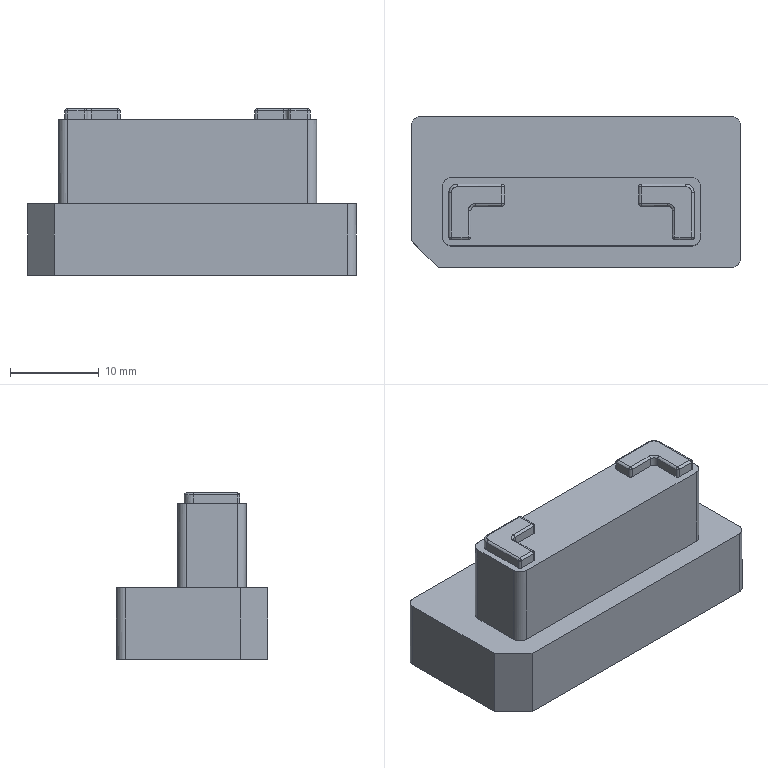NC program | PowerMill | posted with a generic post | part box 37 x 17 x 18.689 mm
Lines 5651 to 6708 of 30982:
N5748 M6
N5749 S18000 M03
N5750 G00 G90 X0.0 Y0.0
N5751 G43 Z10.799 H10
N5752
N5753 G05 P10000 R8
N5754 X9.3537 Y2.5995
N5755 Z0.909
N5756 G01 Z-0.291 F1200.0
N5757 X9.3557 Y2.5558 F2000.0
N5758 X9.3616 Y2.5124
N5759 X9.3715 Y2.4698
N5760 X9.3853 Y2.4282
N5761 X9.4027 Y2.3881
N5762 X9.4238 Y2.3497
N5763 X9.4482 Y2.3134
N5764 X9.4758 Y2.2795
N5765 X9.5065 Y2.2483
N5766 X9.5398 Y2.2199
N5767 X9.5756 Y2.1948
N5768 X9.6135 Y2.1729
N5769 X9.6533 Y2.1547
N5770 X9.6945 Y2.1401
N5771 X9.7369 Y2.1293
N5772 X9.7801 Y2.1225
N5773 X9.8238 Y2.1196
N5774 X9.8337 Y2.1195
N5775 X11.5051 Y2.1194
N5776 X12.1964 Y2.1195
N5777 X12.2661 Y2.1196
N5778 X12.3358 Y2.1193
N5779 X12.4054 Y2.1178
N5780 X12.4749 Y2.1141
N5781 X12.5442 Y2.1081
N5782 X12.6133 Y2.0999
N5783 X12.6822 Y2.0897
N5784 X12.7708 Y2.0731
N5785 X12.8612 Y2.0522
N5786 X12.9524 Y2.0271
N5787 X13.0432 Y1.9979
N5788 X13.1315 Y1.9654
N5789 X13.2164 Y1.9301
N5790 X13.2974 Y1.8924
N5791 X13.3816 Y1.8488
N5792 X13.4635 Y1.8021
N5793 X13.543 Y1.7523
N5794 X13.6202 Y1.6991
N5795 X13.6951 Y1.6427
N5796 X13.7679 Y1.5829
N5797 X13.8384 Y1.5198
N5798 X13.905 Y1.4552
N5799 X13.9691 Y1.3876
N5800 X14.0308 Y1.3168
N5801 X14.09 Y1.2429
N5802 X14.143 Y1.1708
N5803 X14.1929 Y1.0965
N5804 X14.2412 Y1.0177
N5805 X14.2873 Y0.9351
N5806 X14.3304 Y0.8495
N5807 X14.3697 Y0.7626
N5808 X14.4047 Y0.6758
N5809 X14.4353 Y0.59
N5810 X14.4617 Y0.5046
N5811 X14.4847 Y0.4181
N5812 X14.5061 Y0.3236
N5813 X14.5231 Y0.2313
N5814 X14.5359 Y0.141
N5815 X14.5434 Y0.0647
N5816 X14.5479 Y-0.0169
N5817 X14.5497 Y-0.116
N5818 X14.5499 Y-0.1999
N5819 X14.5496 Y-2.5992
N5820 X14.5499 Y-4.1425
N5821 X14.5505 Y-4.9985
N5822 X14.5502 Y-5.0629
N5823 X14.5489 Y-5.1274
N5824 X14.5457 Y-5.1946
N5825 X14.5397 Y-5.2666
N5826 X14.5302 Y-5.3388
N5827 X14.5182 Y-5.4041
N5828 X14.5037 Y-5.4667
N5829 X14.4864 Y-5.5287
N5830 X14.4615 Y-5.6043
N5831 X14.4329 Y-5.6785
N5832 X14.4006 Y-5.7512
N5833 X14.3666 Y-5.8187
N5834 X14.329 Y-5.8846
N5835 X14.2874 Y-5.9495
N5836 X14.242 Y-6.0131
N5837 X14.193 Y-6.0747
N5838 X14.1411 Y-6.1337
N5839 X14.0866 Y-6.1895
N5840 X14.0301 Y-6.2418
N5841 X13.9717 Y-6.2906
N5842 X13.9086 Y-6.3382
N5843 X13.8441 Y-6.382
N5844 X13.7782 Y-6.422
N5845 X13.7112 Y-6.458
N5846 X13.6426 Y-6.4907
N5847 X13.5709 Y-6.5208
N5848 X13.5007 Y-6.5462
N5849 X13.432 Y-6.567
N5850 X13.3723 Y-6.5819
N5851 X13.3121 Y-6.5947
N5852 X13.2516 Y-6.6053
N5853 X13.1906 Y-6.6132
N5854 X13.124 Y-6.6189
N5855 X13.0569 Y-6.6218
N5856 X12.9952 Y-6.623
N5857 X12.9335 Y-6.6233
N5858 X12.8718
N5859 X12.0465
N5860 X11.525 Y-6.623
N5861 X11.1967 Y-6.6245
N5862 X11.1288 Y-6.6246
N5863 X11.0609 Y-6.6232
N5864 X10.9905 Y-6.6194
N5865 X10.9202 Y-6.6125
N5866 X10.8531 Y-6.6026
N5867 X10.7864 Y-6.5896
N5868 X10.709 Y-6.5709
N5869 X10.6333 Y-6.5484
N5870 X10.5596 Y-6.5225
N5871 X10.488 Y-6.4931
N5872 X10.4186 Y-6.4604
N5873 X10.3517 Y-6.4245
N5874 X10.287 Y-6.3853
N5875 X10.2207 Y-6.3405
N5876 X10.1571 Y-6.2928
N5877 X10.0964 Y-6.2422
N5878 X10.0387 Y-6.1889
N5879 X9.984 Y-6.1331
N5880 X9.9324 Y-6.0748
N5881 X9.8841 Y-6.0142
N5882 X9.839 Y-5.9512
N5883 X9.7972 Y-5.8859
N5884 X9.7583 Y-5.8179
N5885 X9.7229 Y-5.7479
N5886 X9.6912 Y-5.6763
N5887 X9.6631 Y-5.603
N5888 X9.6387 Y-5.5283
N5889 X9.6182 Y-5.4525
N5890 X9.6015 Y-5.3756
N5891 X9.5909 Y-5.3131
N5892 X9.5831 Y-5.2502
N5893 X9.5782 Y-5.187
N5894 X9.5756 Y-5.1138
N5895 X9.575 Y-5.0502
N5896 X9.5749 Y-4.9867
N5897 X9.5755 Y-3.0945
N5898 X9.5735 Y-3.0638
N5899 X9.5676 Y-3.0336
N5900 X9.5578 Y-3.0042
N5901 X9.5443 Y-2.9763
N5902 X9.5275 Y-2.9505
N5903 X9.5075 Y-2.9272
N5904 X9.4846 Y-2.9065
N5905 X9.4594 Y-2.889
N5906 X9.432 Y-2.8748
N5907 X9.403 Y-2.8642
N5908 X9.3728 Y-2.8575
N5909 X9.3421 Y-2.8546
N5910 X9.3355 Y-2.8545
N5911 X8.1434 Y-2.8546
N5912 X7.3978 Y-2.8551
N5913 X7.3348 Y-2.8547
N5914 X7.2718 Y-2.8528
N5915 X7.2089 Y-2.8492
N5916 X7.1462 Y-2.8432
N5917 X7.0839 Y-2.8345
N5918 X7.0209 Y-2.8225
N5919 X6.955 Y-2.8063
N5920 X6.8944 Y-2.7886
N5921 X6.8345 Y-2.7689
N5922 X6.7751 Y-2.7477
N5923 X6.7116 Y-2.7215
N5924 X6.6468 Y-2.6905
N5925 X6.5804 Y-2.6545
N5926 X6.5122 Y-2.6131
N5927 X6.4473 Y-2.5693
N5928 X6.385 Y-2.5225
N5929 X6.3254 Y-2.4728
N5930 X6.2686 Y-2.4202
N5931 X6.2146 Y-2.3649
N5932 X6.1636 Y-2.3068
N5933 X6.1155 Y-2.2461
N5934 X6.0695 Y-2.1817
N5935 X6.0269 Y-2.1154
N5936 X5.9881 Y-2.0476
N5937 X5.9533 Y-1.9789
N5938 X5.9226 Y-1.9096
N5939 X5.8959 Y-1.8399
N5940 X5.871 Y-1.7635
N5941 X5.8506 Y-1.6891
N5942 X5.8346 Y-1.6162
N5943 X5.8252 Y-1.5623
N5944 X5.8173 Y-1.5083
N5945 X5.8115 Y-1.454
N5946 X5.8079 Y-1.3995
N5947 X5.8063 Y-1.3401
N5948 Y-1.2852
N5949 X5.8066 Y-1.2304
N5950 X5.8067 Y-1.1757
N5951 X5.8064 Y-0.3499
N5952 X5.8068 Y0.1875
N5953 X5.8057 Y0.4998
N5954 X5.8061 Y0.6018
N5955 X5.8092 Y0.6844
N5956 X5.8152 Y0.7564
N5957 X5.8243 Y0.8235
N5958 X5.8388 Y0.902
N5959 X5.8569 Y0.9783
N5960 X5.8784 Y1.0523
N5961 X5.9035 Y1.1243
N5962 X5.933 Y1.197
N5963 X5.9661 Y1.2682
N5964 X6.0029 Y1.3376
N5965 X6.0431 Y1.405
N5966 X6.0867 Y1.4703
N5967 X6.1335 Y1.5333
N5968 X6.1834 Y1.5937
N5969 X6.2363 Y1.6515
N5970 X6.292 Y1.7064
N5971 X6.3503 Y1.7583
N5972 X6.4112 Y1.8072
N5973 X6.4744 Y1.8528
N5974 X6.5399 Y1.8952
N5975 X6.5975 Y1.9283
N5976 X6.6656 Y1.9633
N5977 X6.7429 Y2.0003
N5978 X6.7709 Y2.0122
N5979 X6.7995 Y2.0229
N5980 X6.8298 Y2.0334
N5981 X6.8684 Y2.046
N5982 X6.9207 Y2.0618
N5983 X6.9785 Y2.0775
N5984 X7.0208 Y2.0875
N5985 X7.0543 Y2.0943
N5986 X7.0844 Y2.0989
N5987 X7.1147 Y2.103
N5988 X7.163 Y2.1105
N5989 X7.1969 Y2.1138
N5990 X7.2308 Y2.1157
N5991 X7.2811 Y2.1191
N5992 X7.3316 Y2.1203
N5993 X7.4192 Y2.1198
N5994 X7.518 Y2.1196
N5995 X7.8845 Y2.1195
N5996 X9.8337
N5997 X9.8774 Y2.1215
N5998 X9.9207 Y2.1274
N5999 X9.9633 Y2.1373
N6000 X10.0049 Y2.151
N6001 X10.045 Y2.1685
N6002 X10.0834 Y2.1895
N6003 X10.1197 Y2.214
N6004 X10.1536 Y2.2416
N6005 X10.1849 Y2.2723
N6006 X10.2132 Y2.3056
N6007 X10.2384 Y2.3414
N6008 X10.2602 Y2.3793
N6009 X10.2785 Y2.4191
N6010 X10.2931 Y2.4603
N6011 X10.3038 Y2.5027
N6012 X10.3107 Y2.5459
N6013 X10.3136 Y2.5896
N6014 X10.3137 Y2.5995
N6015 X9.3537 Y2.6417 Z-0.311
N6016 X9.3557 Y2.598
N6017 X9.3616 Y2.5547
N6018 X9.3715 Y2.512
N6019 X9.3853 Y2.4705
N6020 X9.4027 Y2.4303
N6021 X9.4238 Y2.392
N6022 X9.4482 Y2.3557
N6023 X9.4759 Y2.3218
N6024 X9.5065 Y2.2905
N6025 X9.5398 Y2.2622
N6026 X9.5756 Y2.237
N6027 X9.6135 Y2.2152
N6028 X9.6533 Y2.1969
N6029 X9.6945 Y2.1823
N6030 X9.7369 Y2.1715
N6031 X9.7801 Y2.1647
N6032 X9.8238 Y2.1618
N6033 X9.8337 Y2.1617
N6034 X11.0185 Y2.1616
N6035 X12.1273 Y2.1622
N6036 X12.2964 Y2.1625
N6037 X12.3945 Y2.1607
N6038 X12.4917 Y2.155
N6039 X12.5879 Y2.1454
N6040 X12.6829 Y2.1319
N6041 X12.7764 Y2.1147
N6042 X12.8685 Y2.0936
N6043 X12.9595 Y2.0688
N6044 X13.0504 Y2.0399
N6045 X13.1399 Y2.0072
N6046 X13.228 Y1.9708
N6047 X13.3145 Y1.9308
N6048 X13.3992 Y1.8871
N6049 X13.4822 Y1.8398
N6050 X13.5631 Y1.7891
N6051 X13.6419 Y1.7351
N6052 X13.7183 Y1.6778
N6053 X13.7922 Y1.6174
N6054 X13.8636 Y1.5539
N6055 X13.9322 Y1.4875
N6056 X13.998 Y1.4183
N6057 X14.0609 Y1.3464
N6058 X14.1207 Y1.2719
N6059 X14.1773 Y1.195
N6060 X14.2305 Y1.1159
N6061 X14.2804 Y1.0347
N6062 X14.3267 Y0.9516
N6063 X14.3694 Y0.8669
N6064 X14.4084 Y0.7808
N6065 X14.4435 Y0.6934
N6066 X14.4748 Y0.605
N6067 X14.5023 Y0.5156
N6068 X14.5279 Y0.4191
N6069 X14.5488 Y0.3262
N6070 X14.5652 Y0.2361
N6071 X14.5772 Y0.1487
N6072 X14.5852 Y0.0628
N6073 X14.5898 Y-0.0285
N6074 X14.5918 Y-0.1377
N6075 X14.5917 Y-0.2938
N6076 Y-0.5033
N6077 Y-2.8628
N6078 X14.5925 Y-4.9985
N6079 X14.5922 Y-5.0621
N6080 X14.591 Y-5.1257
N6081 X14.5883 Y-5.1892
N6082 X14.5832 Y-5.2569
N6083 X14.5743 Y-5.33
N6084 X14.5631 Y-5.3948
N6085 X14.5495 Y-5.4567
N6086 X14.5334 Y-5.5181
N6087 X14.5105 Y-5.5913
N6088 X14.4829 Y-5.6664
N6089 X14.4528 Y-5.7381
N6090 X14.4189 Y-5.8087
N6091 X14.381 Y-5.8782
N6092 X14.3392 Y-5.9467
N6093 X14.2964 Y-6.0099
N6094 X14.2504 Y-6.071
N6095 X14.2007 Y-6.1305
N6096 X14.1473 Y-6.1881
N6097 X14.0907 Y-6.2434
N6098 X14.0309 Y-6.2962
N6099 X13.9684 Y-6.3461
N6100 X13.9035 Y-6.3928
N6101 X13.8367 Y-6.4359
N6102 X13.7684 Y-6.4753
N6103 X13.699 Y-6.5108
N6104 X13.6282 Y-6.5427
N6105 X13.5556 Y-6.5713
N6106 X13.4833 Y-6.5956
N6107 X13.4113 Y-6.6157
N6108 X13.3524 Y-6.6295
N6109 X13.2931 Y-6.6414
N6110 X13.2336 Y-6.6512
N6111 X13.1736 Y-6.6585
N6112 X13.1133 Y-6.6632
N6113 X13.0392 Y-6.6657
N6114 X12.9786 Y-6.6661
N6115 X12.9179 Y-6.6659
N6116 X12.8574 Y-6.6657
N6117 X12.2011 Y-6.6654
N6118 X11.1967
N6119 X11.1326 Y-6.6651
N6120 X11.0646 Y-6.6639
N6121 X10.9895 Y-6.6604
N6122 X10.9149 Y-6.6538
N6123 X10.8496 Y-6.6449
N6124 X10.7868 Y-6.6333
N6125 X10.7246 Y-6.6189
N6126 X10.6629 Y-6.6019
N6127 X10.5866 Y-6.5771
N6128 X10.5119 Y-6.5487
N6129 X10.4388 Y-6.5166
N6130 X10.3676 Y-6.481
N6131 X10.2984 Y-6.4419
N6132 X10.2314 Y-6.3995
N6133 X10.1667 Y-6.3538
N6134 X10.1045 Y-6.305
N6135 X10.0448 Y-6.2531
N6136 X9.9883 Y-6.1987
N6137 X9.9345 Y-6.1416
N6138 X9.8836 Y-6.0817
N6139 X9.8355 Y-6.0188
N6140 X9.7902 Y-5.9532
N6141 X9.7479 Y-5.8849
N6142 X9.7087 Y-5.8139
N6143 X9.6753 Y-5.7459
N6144 X9.6452 Y-5.6757
N6145 X9.6185 Y-5.6031
N6146 X9.595 Y-5.5281
N6147 X9.5777 Y-5.4623
N6148 X9.5629 Y-5.396
N6149 X9.5509 Y-5.329
N6150 X9.542 Y-5.2616
N6151 X9.5359 Y-5.1901
N6152 X9.5326 Y-5.1108
N6153 X9.5319 Y-5.0426
N6154 X9.5323 Y-4.9745
N6155 X9.5337 Y-4.6149
N6156 X9.5334 Y-4.171
N6157 Y-3.1367
N6158 X9.5314 Y-3.1058
N6159 X9.5254 Y-3.0755
N6160 X9.5157 Y-3.0462
N6161 X9.5022 Y-3.0184
N6162 X9.4852 Y-2.9925
N6163 X9.4652 Y-2.9691
N6164 X9.4424 Y-2.9485
N6165 X9.4171 Y-2.931
N6166 X9.3898 Y-2.9169
N6167 X9.3607 Y-2.9063
N6168 X9.3306 Y-2.8995
N6169 X9.2999 Y-2.8967
N6170 X9.2934 Y-2.8966
N6171 X8.2956 Y-2.8967
N6172 X7.6583 Y-2.8969
N6173 X7.2979 Y-2.8957
N6174 X7.23 Y-2.8933
N6175 X7.1616 Y-2.8874
N6176 X7.0888 Y-2.8775
N6177 X7.0125 Y-2.8633
N6178 X6.9347 Y-2.8448
N6179 X6.86 Y-2.823
N6180 X6.7917 Y-2.7995
N6181 X6.7195 Y-2.7705
N6182 X6.6481 Y-2.7375
N6183 X6.5775 Y-2.7006
N6184 X6.5079 Y-2.6597
N6185 X6.4394 Y-2.6148
N6186 X6.3774 Y-2.5698
N6187 X6.3174 Y-2.5213
N6188 X6.2594 Y-2.4695
N6189 X6.2038 Y-2.4143
N6190 X6.1506 Y-2.356
N6191 X6.1001 Y-2.2947
N6192 X6.0526 Y-2.2307
N6193 X6.0082 Y-2.1642
N6194 X5.9671 Y-2.0955
N6195 X5.9295 Y-2.025
N6196 X5.8963 Y-1.9542
N6197 X5.8666 Y-1.8819
N6198 X5.8406 Y-1.808
N6199 X5.8182 Y-1.7325
N6200 X5.7997 Y-1.6557
N6201 X5.7886 Y-1.5993
N6202 X5.7794 Y-1.5426
N6203 X5.7723 Y-1.4857
N6204 X5.7674 Y-1.4285
N6205 X5.7649 Y-1.3711
N6206 X5.7641 Y-1.3052
N6207 X5.7643 Y-1.2476
N6208 X5.7645 Y-1.1901
N6209 X5.7646 Y-0.3499
N6210 X5.7647 Y0.2261
N6211 X5.7638 Y0.4998
N6212 X5.7637 Y0.5597
N6213 X5.7644 Y0.6195
N6214 X5.7666 Y0.6793
N6215 X5.7711 Y0.7389
N6216 X5.7782 Y0.7983
N6217 X5.7877 Y0.8573
N6218 X5.799 Y0.916
N6219 X5.8167 Y0.991
N6220 X5.8384 Y1.0655
N6221 X5.864 Y1.1393
N6222 X5.8936 Y1.2122
N6223 X5.9269 Y1.2841
N6224 X5.964 Y1.3545
N6225 X6.0046 Y1.423
N6226 X6.0486 Y1.4894
N6227 X6.0959 Y1.5535
N6228 X6.1463 Y1.6151
N6229 X6.1996 Y1.6741
N6230 X6.2558 Y1.7301
N6231 X6.3146 Y1.7832
N6232 X6.3758 Y1.8332
N6233 X6.4394 Y1.88
N6234 X6.5052 Y1.9234
N6235 X6.5731 Y1.9634
N6236 X6.6421 Y1.9995
N6237 X6.7133 Y2.0324
N6238 X6.7874 Y2.0622
N6239 X6.8644 Y2.0888
N6240 X6.9354 Y2.1098
N6241 X7.0072 Y2.127
N6242 X7.0799 Y2.1405
N6243 X7.1562 Y2.1509
N6244 X7.2379 Y2.158
N6245 X7.3262 Y2.1619
N6246 X7.423 Y2.1627
N6247 X8.5939 Y2.1618
N6248 X9.8337 Y2.1617
N6249 X9.8774 Y2.1637
N6250 X9.9207 Y2.1697
N6251 X9.9633 Y2.1795
N6252 X10.0049 Y2.1933
N6253 X10.045 Y2.2107
N6254 X10.0834 Y2.2318
N6255 X10.1197 Y2.2562
N6256 X10.1536 Y2.2839
N6257 X10.1849 Y2.3145
N6258 X10.2132 Y2.3478
N6259 X10.2384 Y2.3836
N6260 X10.2602 Y2.4215
N6261 X10.2785 Y2.4613
N6262 X10.2931 Y2.5025
N6263 X10.3038 Y2.5449
N6264 X10.3107 Y2.5881
N6265 X10.3136 Y2.6318
N6266 X10.3137 Y2.6417
N6267 X9.3536 Y2.6722 Z-0.331
N6268 X9.3556 Y2.6285
N6269 X9.3616 Y2.5851
N6270 X9.3715 Y2.5425
N6271 X9.3852 Y2.5009
N6272 X9.4027 Y2.4608
N6273 X9.4237 Y2.4224
N6274 X9.4482 Y2.3861
N6275 X9.4758 Y2.3522
N6276 X9.5064 Y2.321
N6277 X9.5398 Y2.2927
N6278 X9.5755 Y2.2675
N6279 X9.6135 Y2.2457
N6280 X9.6533 Y2.2274
N6281 X9.6945 Y2.2128
N6282 X9.7369 Y2.2021
N6283 X9.7801 Y2.1952
N6284 X9.8238 Y2.1923
N6285 X9.8337 Y2.1922
N6286 X10.956 Y2.1924
N6287 X12.2964 Y2.1923
N6288 X12.3993 Y2.1904
N6289 X12.4979 Y2.1848
N6290 X12.5925 Y2.1757
N6291 X12.6835 Y2.1631
N6292 X12.7713 Y2.1472
N6293 X12.8578 Y2.1276
N6294 X12.9526 Y2.1024
N6295 X13.0446 Y2.0739
N6296 X13.1339 Y2.0421
N6297 X13.2205 Y2.0072
N6298 X13.3053 Y1.9689
N6299 X13.3917 Y1.9255
N6300 X13.4757 Y1.8789
N6301 X13.5573 Y1.8292
N6302 X13.6365 Y1.7762
N6303 X13.7141 Y1.7195
N6304 X13.7893 Y1.6596
N6305 X13.8619 Y1.5967
N6306 X13.9318 Y1.5308
N6307 X13.9989 Y1.462
N6308 X14.0632 Y1.3905
N6309 X14.1244 Y1.3164
N6310 X14.1825 Y1.2398
N6311 X14.2373 Y1.1608
N6312 X14.2888 Y1.0797
N6313 X14.3369 Y0.9965
N6314 X14.3815 Y0.9114
N6315 X14.422 Y0.8254
N6316 X14.4593 Y0.7372
N6317 X14.4929 Y0.647
N6318 X14.523 Y0.5553
N6319 X14.5492 Y0.4625
N6320 X14.5714 Y0.369
N6321 X14.5896 Y0.2751
N6322 X14.6039 Y0.1812
N6323 X14.614 Y0.0877
N6324 X14.6202 Y-0.0052
N6325 X14.6223 Y-0.0972
N6326 Y-0.1892
N6327 Y-2.9242
N6328 Y-3.7207
N6329 X14.6221 Y-4.5754
N6330 X14.6232 Y-4.9985
N6331 X14.6231 Y-5.0648
N6332 X14.6218 Y-5.1311
N6333 X14.6188 Y-5.1974
N6334 X14.6132 Y-5.2652
N6335 X14.6048 Y-5.3309
N6336 X14.5936 Y-5.3962
N6337 X14.5797 Y-5.461
N6338 X14.5596 Y-5.537
N6339 X14.5355 Y-5.6127
N6340 X14.5074 Y-5.6878
N6341 X14.4753 Y-5.7622
N6342 X14.4401 Y-5.8342
N6343 X14.4015 Y-5.9039
N6344 X14.3597 Y-5.9715
N6345 X14.3146 Y-6.0368
N6346 X14.2662 Y-6.0997
N6347 X14.2147 Y-6.1603
N6348 X14.16 Y-6.2185
N6349 X14.1021 Y-6.2741
N6350 X14.0411 Y-6.3272
N6351 X13.9771 Y-6.3777
N6352 X13.9141 Y-6.4227
N6353 X13.8486 Y-6.4647
N6354 X13.7804 Y-6.5036
N6355 X13.7097 Y-6.5395
N6356 X13.6365 Y-6.5721
N6357 X13.561 Y-6.6014
N6358 X13.4866 Y-6.6262
N6359 X13.411 Y-6.6474
N6360 X13.3338 Y-6.6649
N6361 X13.255 Y-6.6787
N6362 X13.1749 Y-6.6886
N6363 X13.0936 Y-6.6947
N6364 X13.0114 Y-6.6969
N6365 X12.9285 Y-6.6965
N6366 X12.5012 Y-6.6959
N6367 X11.758 Y-6.6964
N6368 X11.1967 Y-6.6969
N6369 X11.1223 Y-6.6964
N6370 X11.0452 Y-6.694
N6371 X10.9651 Y-6.6889
N6372 X10.8859 Y-6.6804
N6373 X10.8127 Y-6.6689
N6374 X10.7446 Y-6.6548
N6375 X10.6787 Y-6.638
N6376 X10.6136 Y-6.6183
N6377 X10.5492 Y-6.5959
N6378 X10.4746 Y-6.5661
N6379 X10.4018 Y-6.5327
N6380 X10.3311 Y-6.4959
N6381 X10.2625 Y-6.4557
N6382 X10.1959 Y-6.4121
N6383 X10.1307 Y-6.3646
N6384 X10.0681 Y-6.3141
N6385 X10.0083 Y-6.2606
N6386 X9.9511 Y-6.2042
N6387 X9.8971 Y-6.1453
N6388 X9.847 Y-6.0849
N6389 X9.7997 Y-6.0216
N6390 X9.7552 Y-5.9554
N6391 X9.7134 Y-5.8861
N6392 X9.6745 Y-5.8139
N6393 X9.642 Y-5.746
N6394 X9.6126 Y-5.6754
N6395 X9.586 Y-5.6013
N6396 X9.5648 Y-5.5328
N6397 X9.5465 Y-5.4636
N6398 X9.5313 Y-5.3936
N6399 X9.5194 Y-5.3228
N6400 X9.5103 Y-5.2468
N6401 X9.5042 Y-5.1644
N6402 X9.5014 Y-5.0773
N6403 X9.5013 Y-4.9985
N6404 X9.503 Y-4.6794
N6405 X9.5027 Y-4.2175
N6406 Y-3.6648
N6407 Y-3.1673
N6408 X9.5007 Y-3.1365
N6409 X9.4948 Y-3.1061
N6410 X9.485 Y-3.0768
N6411 X9.4715 Y-3.049
N6412 X9.4546 Y-3.0231
N6413 X9.4346 Y-2.9998
N6414 X9.4118 Y-2.9792
N6415 X9.3865 Y-2.9617
N6416 X9.3592 Y-2.9475
N6417 X9.3301 Y-2.9369
N6418 X9.3226 Y-2.9353
N6419 X9.2999 Y-2.9302
N6420 X9.2692 Y-2.9274
N6421 X9.2627 Y-2.9273
N6422 X8.3356 Y-2.9271
N6423 X7.4084 Y-2.9264
N6424 X7.2979 Y-2.9262
N6425 X7.2263 Y-2.924
N6426 X7.1537 Y-2.9179
N6427 X7.08 Y-2.9077
N6428 X7.005 Y-2.8933
N6429 X6.929 Y-2.8747
N6430 X6.8517 Y-2.8518
N6431 X6.7734 Y-2.8244
N6432 X6.6981 Y-2.7942
N6433 X6.6335 Y-2.7647
N6434 X6.5668 Y-2.7299
N6435 X6.4981 Y-2.6897
N6436 X6.431 Y-2.6461
N6437 X6.3662 Y-2.5993
N6438 X6.3038 Y-2.5492
N6439 X6.2439 Y-2.4961
N6440 X6.1868 Y-2.4401
N6441 X6.1325 Y-2.3813
N6442 X6.0812 Y-2.3198
N6443 X6.033 Y-2.2558
N6444 X5.988 Y-2.1895
N6445 X5.9465 Y-2.1211
N6446 X5.9084 Y-2.0507
N6447 X5.8739 Y-1.9785
N6448 X5.843 Y-1.9047
N6449 X5.8158 Y-1.8295
N6450 X5.7927 Y-1.7541
N6451 X5.7734 Y-1.6773
N6452 X5.7577 Y-1.5989
N6453 X5.7458 Y-1.5191
N6454 X5.7378 Y-1.4381
N6455 X5.7337 Y-1.3561
N6456 X5.7333 Y-1.2732
N6457 X5.7341 Y-0.8651
N6458 X5.7337 Y-0.1581
N6459 X5.7332 Y0.4999
N6460 X5.7336 Y0.5681
N6461 X5.7354 Y0.64
N6462 X5.7398 Y0.7171
N6463 X5.7474 Y0.7947
N6464 X5.7577 Y0.8645
N6465 X5.7706 Y0.9303
N6466 X5.7864 Y0.9956
N6467 X5.805 Y1.0602
N6468 X5.8304 Y1.1359
N6469 X5.8596 Y1.2102
N6470 X5.8924 Y1.283
N6471 X5.9288 Y1.3541
N6472 X5.9687 Y1.4233
N6473 X6.012 Y1.4905
N6474 X6.0586 Y1.5555
N6475 X6.1085 Y1.6182
N6476 X6.1615 Y1.6783
N6477 X6.2174 Y1.7357
N6478 X6.276 Y1.7902
N6479 X6.3373 Y1.8417
N6480 X6.401 Y1.89
N6481 X6.467 Y1.9351
N6482 X6.5351 Y1.9768
N6483 X6.6052 Y2.015
N6484 X6.6771 Y2.0497
N6485 X6.7506 Y2.0808
N6486 X6.8257 Y2.1083
N6487 X6.9031 Y2.1325
N6488 X6.9803 Y2.1526
N6489 X7.0566 Y2.1684
N6490 X7.1312 Y2.1801
N6491 X7.2039 Y2.1875
N6492 X7.2745 Y2.1909
N6493 X7.3442 Y2.1913
N6494 X8.5123 Y2.1921
N6495 X9.8337 Y2.1922
N6496 X9.8774 Y2.1942
N6497 X9.9207 Y2.2002
N6498 X9.9633 Y2.2101
N6499 X10.0049 Y2.2238
N6500 X10.045 Y2.2413
N6501 X10.0834 Y2.2624
N6502 X10.1197 Y2.2868
N6503 X10.1536 Y2.3145
N6504 X10.1848 Y2.3451
N6505 X10.2132 Y2.3784
N6506 X10.2383 Y2.4142
N6507 X10.2601 Y2.4521
N6508 X10.2784 Y2.4919
N6509 X10.293 Y2.5332
N6510 X10.3038 Y2.5756
N6511 X10.3106 Y2.6188
N6512 X10.3135 Y2.6624
N6513 X10.3136 Y2.6723
N6514 X9.3536 Y2.6962 Z-0.351
N6515 X9.3556 Y2.6525
N6516 X9.3616 Y2.6091
N6517 X9.3715 Y2.5665
N6518 X9.3852 Y2.5249
N6519 X9.4027 Y2.4848
N6520 X9.4237 Y2.4464
N6521 X9.4482 Y2.4101
N6522 X9.4758 Y2.3762
N6523 X9.5064 Y2.345
N6524 X9.5398 Y2.3167
N6525 X9.5755 Y2.2915
N6526 X9.6135 Y2.2697
N6527 X9.6533 Y2.2514
N6528 X9.6945 Y2.2368
N6529 X9.7369 Y2.2261
N6530 X9.7801 Y2.2192
N6531 X9.8238 Y2.2163
N6532 X9.8337 Y2.2162
N6533 X10.859 Y2.2164
N6534 X12.1965 Y2.217
N6535 X12.2764 Y2.2167
N6536 X12.3565 Y2.2155
N6537 X12.4385 Y2.2125
N6538 X12.53 Y2.2062
N6539 X12.6094 Y2.1976
N6540 X12.6884 Y2.1862
N6541 X12.767 Y2.172
N6542 X12.8452 Y2.1552
N6543 X12.9383 Y2.1315
N6544 X13.0303 Y2.1039
N6545 X13.1211 Y2.0726
N6546 X13.2107 Y2.0374
N6547 X13.2988 Y1.9985
N6548 X13.3854 Y1.956
N6549 X13.4704 Y1.9097
N6550 X13.5533 Y1.8601
N6551 X13.6341 Y1.8071
N6552 X13.7126 Y1.7508
N6553 X13.7886 Y1.6914
N6554 X13.862 Y1.6289
N6555 X13.9327 Y1.5635
N6556 X14.0006 Y1.4952
N6557 X14.066 Y1.4238
N6558 X14.1283 Y1.3499
N6559 X14.1874 Y1.2736
N6560 X14.2433 Y1.195
N6561 X14.2958 Y1.1142
N6562 X14.345 Y1.0312
N6563 X14.3907 Y0.9462
N6564 X14.4329 Y0.8593
N6565 X14.4715 Y0.7706
N6566 X14.5058 Y0.6822
N6567 X14.5366 Y0.5919
N6568 X14.564 Y0.4994
N6569 X14.5877 Y0.4054
N6570 X14.6074 Y0.3108
N6571 X14.6231 Y0.216
N6572 X14.6347 Y0.1217
N6573 X14.6423 Y0.0283
N6574 X14.6459 Y-0.0637
N6575 X14.6462 Y-0.1552
N6576 X14.6463 Y-3.7207
N6577 X14.6468 Y-4.642
N6578 X14.6476 Y-4.9985
N6579 X14.6473 Y-5.0644
N6580 X14.6459 Y-5.1302
N6581 X14.6428 Y-5.1961
N6582 X14.6375 Y-5.2617
N6583 X14.6283 Y-5.3344
N6584 X14.6171 Y-5.3992
N6585 X14.6033 Y-5.4636
N6586 X14.5873 Y-5.5274
N6587 X14.5659 Y-5.5983
N6588 X14.5398 Y-5.6712
N6589 X14.5087 Y-5.7466
N6590 X14.4753 Y-5.8181
N6591 X14.4384 Y-5.8882
N6592 X14.3977 Y-5.9567
N6593 X14.3533 Y-6.0237
N6594 X14.3053 Y-6.0888
N6595 X14.2539 Y-6.152
N6596 X14.199 Y-6.2131
N6597 X14.1462 Y-6.2663
N6598 X14.0888 Y-6.3186
N6599 X14.0257 Y-6.3707
N6600 X13.9633 Y-6.4178
N6601 X13.8985 Y-6.462
N6602 X13.8311 Y-6.503
N6603 X13.7612 Y-6.541
N6604 X13.6889 Y-6.5756
N6605 X13.6145 Y-6.6069
N6606 X13.5381 Y-6.6348
N6607 X13.4598 Y-6.659
N6608 X13.385 Y-6.6784
N6609 X13.3091 Y-6.6941
N6610 X13.2308 Y-6.7063
N6611 X13.1501 Y-6.7149
N6612 X13.067 Y-6.7197
N6613 X12.9815 Y-6.7208
N6614 X12.2241 Y-6.7201
N6615 X11.1967 Y-6.72
N6616 X11.1326 Y-6.7198
N6617 X11.0684 Y-6.7186
N6618 X11.0006 Y-6.7158
N6619 X10.924 Y-6.7097
N6620 X10.8577 Y-6.7013
N6621 X10.7947 Y-6.6903
N6622 X10.7322 Y-6.6766
N6623 X10.6702 Y-6.6604
N6624 X10.5924 Y-6.6367
N6625 X10.5166 Y-6.6094
N6626 X10.4428 Y-6.5787
N6627 X10.3709 Y-6.5445
N6628 X10.3008 Y-6.5068
N6629 X10.2326 Y-6.4655
N6630 X10.1661 Y-6.4206
N6631 X10.1012 Y-6.3721
N6632 X10.039 Y-6.3207
N6633 X9.9795 Y-6.2665
N6634 X9.9228 Y-6.2094
N6635 X9.869 Y-6.1497
N6636 X9.8183 Y-6.0875
N6637 X9.7708 Y-6.0227
N6638 X9.7264 Y-5.9557
N6639 X9.6854 Y-5.8864
N6640 X9.6479 Y-5.8151
N6641 X9.6138 Y-5.7418
N6642 X9.5833 Y-5.6668
N6643 X9.5592 Y-5.5984
N6644 X9.5388 Y-5.5307
N6645 X9.5212 Y-5.4622
N6646 X9.5075 Y-5.3984
N6647 X9.5042 Y-5.3806
N6648 X9.5011 Y-5.3627
N6649 X9.4962 Y-5.3334
N6650 X9.4935 Y-5.3155
N6651 X9.4914 Y-5.2975
N6652 X9.4839 Y-5.2082
N6653 X9.4793 Y-5.1405
N6654 X9.4784 Y-5.0837
N6655 X9.4787 Y-4.6635
N6656 X9.4786 Y-3.3494
N6657 X9.4787 Y-3.1913
N6658 X9.4767 Y-3.1606
N6659 X9.4708 Y-3.1304
N6660 X9.4611 Y-3.101
N6661 X9.4476 Y-3.0731
N6662 X9.4308 Y-3.0474
N6663 X9.4108 Y-3.024
N6664 X9.388 Y-3.0034
N6665 X9.3627 Y-2.9858
N6666 X9.3353 Y-2.9716
N6667 X9.3123 Y-2.9632
N6668 X9.3063 Y-2.961
N6669 X9.2761 Y-2.9542
N6670 X9.2454 Y-2.9514
N6671 X9.2387 Y-2.9513
N6672 X7.8911 Y-2.951
N6673 X7.2979 Y-2.9501
N6674 X7.224 Y-2.9479
N6675 X7.1504 Y-2.9418
N6676 X7.0766 Y-2.9317
N6677 X7.0018 Y-2.9175
N6678 X6.9261 Y-2.8991
N6679 X6.8492 Y-2.8764
N6680 X6.771 Y-2.8491
N6681 X6.6981 Y-2.8202
N6682 X6.6272 Y-2.7881
N6683 X6.5574 Y-2.7523
N6684 X6.4889 Y-2.7126
N6685 X6.4218 Y-2.6691
N6686 X6.3563 Y-2.622
N6687 X6.2927 Y-2.5712
N6688 X6.2312 Y-2.5171
N6689 X6.1742 Y-2.4619
N6690 X6.12 Y-2.4037
N6691 X6.0684 Y-2.3426
N6692 X6.0197 Y-2.2787
N6693 X5.974 Y-2.2122
N6694 X5.9315 Y-2.1432
N6695 X5.8932 Y-2.0739
N6696 X5.8584 Y-2.0026
N6697 X5.8269 Y-1.9291
N6698 X5.7988 Y-1.8535
N6699 X5.7743 Y-1.7762
N6700 X5.7536 Y-1.6974
N6701 X5.7367 Y-1.6174
N6702 X5.7237 Y-1.5368
N6703 X5.7147 Y-1.4559
N6704 X5.7098 Y-1.375
N6705 X5.7087 Y-1.2943
N6706 X5.7101 Y-0.9606
N6707 X5.7097 Y-0.4998
N6708 X5.71 Y0.4999
N6709 X5.7101 Y0.5561
N6710 X5.7106 Y0.6125
N6711 X5.712 Y0.6687
N6712 X5.7152 Y0.7249
N6713 X5.7209 Y0.7809
N6714 X5.729 Y0.8366
N6715 X5.7384 Y0.892
N6716 X5.7494 Y0.9472
N6717 X5.767 Y1.0175
N6718 X5.7894 Y1.0915
N6719 X5.8168 Y1.1684
N6720 X5.8477 Y1.2438
N6721 X5.8821 Y1.317
N6722 X5.9197 Y1.3879
N6723 X5.9606 Y1.4564
N6724 X6.0048 Y1.5228
N6725 X6.053 Y1.5879
N6726 X6.1043 Y1.6506
N6727 X6.1586 Y1.7105
N6728 X6.2156 Y1.7676
N6729 X6.2753 Y1.8217
N6730 X6.3375 Y1.8727
N6731 X6.4021 Y1.9205
N6732 X6.4698 Y1.9656
N6733 X6.5386 Y2.0068
N6734 X6.6082 Y2.044
N6735 X6.6784 Y2.077
N6736 X6.7494 Y2.1061
N6737 X6.8295 Y2.1348
N6738 X6.9078 Y2.1588
N6739 X6.9846 Y2.1784
N6740 X7.0599 Y2.1937
N6741 X7.1341 Y2.2049
N6742 X7.2073 Y2.2119
N6743 X7.2798 Y2.215
N6744 X7.3525 Y2.2153
N6745 X8.4991 Y2.2161
N6746 X9.8337 Y2.2162
N6747 X9.8774 Y2.2182
N6748 X9.9207 Y2.2242
N6749 X9.9633 Y2.2341
N6750 X10.0049 Y2.2478
N6751 X10.045 Y2.2653
N6752 X10.0834 Y2.2863
N6753 X10.1197 Y2.3108
N6754 X10.1536 Y2.3385
N6755 X10.1848 Y2.3691
N6756 X10.2132 Y2.4024
N6757 X10.2383 Y2.4382
N6758 X10.2601 Y2.4761
N6759 X10.2784 Y2.5159
N6760 X10.293 Y2.5571
N6761 X10.3038 Y2.5996
N6762 X10.3106 Y2.6428
N6763 X10.3135 Y2.6864
N6764 X10.3136 Y2.6963
N6765 X9.3537 Y2.7161 Z-0.371
N6766 X9.3557 Y2.6724
N6767 X9.3616 Y2.6291
N6768 X9.3715 Y2.5864
N6769 X9.3853 Y2.5449
N6770 X9.4027 Y2.5047
N6771 X9.4238 Y2.4664
N6772 X9.4482 Y2.4301
N6773 X9.4758 Y2.3962
N6774 X9.5065 Y2.3649
N6775 X9.5398 Y2.3366
N6776 X9.5756 Y2.3114
N6777 X9.6135 Y2.2896
N6778 X9.6533 Y2.2713
N6779 X9.6945 Y2.2567
N6780 X9.7369 Y2.2459
N6781 X9.7801 Y2.2391
N6782 X9.8238 Y2.2362
N6783 X9.8337 Y2.2361
N6784 X10.8877 Y2.236
N6785 X11.9696 Y2.2367
N6786 X12.1964 Y2.2372
N6787 X12.2846 Y2.2368
N6788 X12.3728 Y2.235
N6789 X12.4609 Y2.231
N6790 X12.5565 Y2.2234
N6791 X12.644 Y2.2131
N6792 X12.7311 Y2.1994
N6793 X12.8194 Y2.1818
N6794 X12.9097 Y2.1597
N6795 X13.0023 Y2.1331
N6796 X13.0974 Y2.1016
N6797 X13.1875 Y2.0679
N6798 X13.2764 Y2.0303
N6799 X13.3636 Y1.9892
N6800 X13.4491 Y1.9444
N6801 X13.5328 Y1.896
N6802 X13.6145 Y1.8442
N6803 X13.6941 Y1.789
N6804 X13.7714 Y1.7305
N6805 X13.8462 Y1.6689